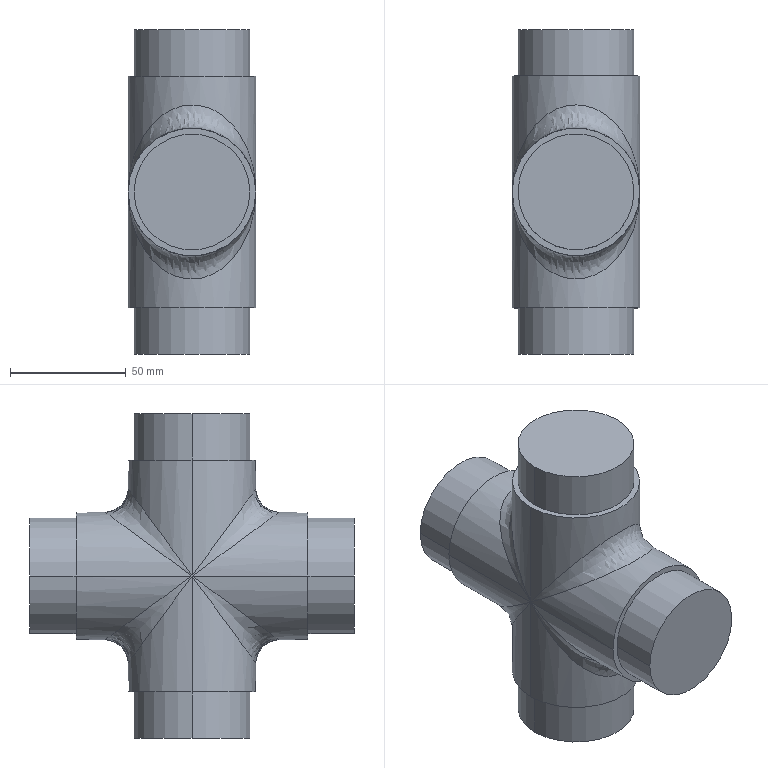Part | SolidWorks | 1 solid | 28 faces | box 55 x 140 x 140 mm | volume 524256 mm3 | cylinder 16 | plane 8 | spline 4 | commonest cylinder face diameters 50 x8 55 x8
STEP:
#1=CARTESIAN_POINT('',(-25.,-70.,0.));
#2=VERTEX_POINT('',#1);
#3=CARTESIAN_POINT('',(25.,-70.,0.));
#4=VERTEX_POINT('',#3);
#5=CARTESIAN_POINT('',(0.,-70.,0.));
#6=DIRECTION('',(0.,1.,0.));
#7=DIRECTION('',(-1.,0.,0.));
#8=AXIS2_PLACEMENT_3D('',#5,#6,#7);
#9=CIRCLE('',#8,25.);
#10=EDGE_CURVE('',#2,#4,#9,.T.);
#11=ORIENTED_EDGE('',*,*,#10,.T.);
#12=CARTESIAN_POINT('',(25.,-50.,0.));
#13=VERTEX_POINT('',#12);
#14=CARTESIAN_POINT('',(25.,70.,0.));
#15=DIRECTION('',(0.,1.,0.));
#16=VECTOR('',#15,1000.);
#17=LINE('',#14,#16);
#18=EDGE_CURVE('',#4,#13,#17,.T.);
#19=ORIENTED_EDGE('',*,*,#18,.T.);
#20=CARTESIAN_POINT('',(-25.,-50.,0.));
#21=VERTEX_POINT('',#20);
#22=CARTESIAN_POINT('',(0.,-50.,0.));
#23=DIRECTION('',(0.,1.,0.));
#24=DIRECTION('',(-1.,0.,0.));
#25=AXIS2_PLACEMENT_3D('',#22,#23,#24);
#26=CIRCLE('',#25,25.);
#27=EDGE_CURVE('',#21,#13,#26,.T.);
#28=ORIENTED_EDGE('',*,*,#27,.F.);
#29=CARTESIAN_POINT('',(-25.,70.,0.));
#30=DIRECTION('',(0.,1.,0.));
#31=VECTOR('',#30,1000.);
#32=LINE('',#29,#31);
#33=EDGE_CURVE('',#2,#21,#32,.T.);
#34=ORIENTED_EDGE('',*,*,#33,.F.);
#35=EDGE_LOOP('',(#11,#19,#28,#34));
#36=FACE_OUTER_BOUND('',#35,.T.);
#37=CARTESIAN_POINT('',(0.,70.,0.));
#38=DIRECTION('',(0.,1.,0.));
#39=DIRECTION('',(-1.,0.,0.));
#40=AXIS2_PLACEMENT_3D('',#37,#38,#39);
#41=CYLINDRICAL_SURFACE('',#40,25.);
#42=ADVANCED_FACE('',(#36),#41,.T.);
#43=CARTESIAN_POINT('',(-27.5,-50.,0.));
#44=VERTEX_POINT('',#43);
#45=CARTESIAN_POINT('',(27.5,-50.,0.));
#46=VERTEX_POINT('',#45);
#47=CARTESIAN_POINT('',(0.,-50.,0.));
#48=DIRECTION('',(0.,1.,0.));
#49=DIRECTION('',(-1.,0.,0.));
#50=AXIS2_PLACEMENT_3D('',#47,#48,#49);
#51=CIRCLE('',#50,27.5);
#52=EDGE_CURVE('',#44,#46,#51,.T.);
#53=ORIENTED_EDGE('',*,*,#52,.T.);
#54=CARTESIAN_POINT('',(27.5,0.,0.));
#55=VERTEX_POINT('',#54);
#56=CARTESIAN_POINT('',(27.5,70.,0.));
#57=DIRECTION('',(0.,1.,0.));
#58=VECTOR('',#57,1000.);
#59=LINE('',#56,#58);
#60=EDGE_CURVE('',#46,#55,#59,.T.);
#61=ORIENTED_EDGE('',*,*,#60,.T.);
#62=CARTESIAN_POINT('',(-27.5,0.,0.));
#63=VERTEX_POINT('',#62);
#64=CARTESIAN_POINT('',(27.5,0.,0.));
#65=CARTESIAN_POINT('',(27.5,-75.,55.));
#66=CARTESIAN_POINT('',(-27.5,-75.,55.));
#67=CARTESIAN_POINT('',(-27.5,0.,0.));
#68=(BOUNDED_CURVE()B_SPLINE_CURVE(3,(#64,#65,#66,#67),.UNSPECIFIED.,.F.,.F.)B_SPLINE_CURVE_WITH_KNOTS((4,4),(1.571,4.712),.UNSPECIFIED.)CURVE()GEOMETRIC_REPRESENTATION_ITEM()RATIONAL_B_SPLINE_CURVE((1.,0.3333,0.3333,1.))REPRESENTATION_ITEM(''));
#69=EDGE_CURVE('',#55,#63,#68,.T.);
#70=ORIENTED_EDGE('',*,*,#69,.T.);
#71=CARTESIAN_POINT('',(-27.5,70.,0.));
#72=DIRECTION('',(0.,1.,0.));
#73=VECTOR('',#72,1000.);
#74=LINE('',#71,#73);
#75=EDGE_CURVE('',#44,#63,#74,.T.);
#76=ORIENTED_EDGE('',*,*,#75,.F.);
#77=EDGE_LOOP('',(#53,#61,#70,#76));
#78=FACE_OUTER_BOUND('',#77,.T.);
#79=CARTESIAN_POINT('',(0.,70.,0.));
#80=DIRECTION('',(0.,1.,0.));
#81=DIRECTION('',(-1.,0.,0.));
#82=AXIS2_PLACEMENT_3D('',#79,#80,#81);
#83=CYLINDRICAL_SURFACE('',#82,27.5);
#84=ADVANCED_FACE('',(#78),#83,.T.);
#85=CARTESIAN_POINT('',(-27.5,0.,0.));
#86=CARTESIAN_POINT('',(-27.5,55.,-75.));
#87=CARTESIAN_POINT('',(27.5,55.,-75.));
#88=CARTESIAN_POINT('',(27.5,0.,0.));
#89=(BOUNDED_CURVE()B_SPLINE_CURVE(3,(#85,#86,#87,#88),.UNSPECIFIED.,.F.,.F.)B_SPLINE_CURVE_WITH_KNOTS((4,4),(4.712,7.854),.UNSPECIFIED.)CURVE()GEOMETRIC_REPRESENTATION_ITEM()RATIONAL_B_SPLINE_CURVE((1.,0.3333,0.3333,1.))REPRESENTATION_ITEM(''));
#90=EDGE_CURVE('',#63,#55,#89,.T.);
#91=ORIENTED_EDGE('',*,*,#90,.T.);
#92=CARTESIAN_POINT('',(27.5,0.,-50.));
#93=VERTEX_POINT('',#92);
#94=CARTESIAN_POINT('',(27.5,0.,50.));
#95=DIRECTION('',(0.,0.,-1.));
#96=VECTOR('',#95,1000.);
#97=LINE('',#94,#96);
#98=EDGE_CURVE('',#55,#93,#97,.T.);
#99=ORIENTED_EDGE('',*,*,#98,.T.);
#100=CARTESIAN_POINT('',(-27.5,0.,-50.));
#101=VERTEX_POINT('',#100);
#102=CARTESIAN_POINT('',(0.,0.,-50.));
#103=DIRECTION('',(0.,0.,1.));
#104=DIRECTION('',(1.,0.,0.));
#105=AXIS2_PLACEMENT_3D('',#102,#103,#104);
#106=CIRCLE('',#105,27.5);
#107=EDGE_CURVE('',#93,#101,#106,.T.);
#108=ORIENTED_EDGE('',*,*,#107,.T.);
#109=CARTESIAN_POINT('',(-27.5,0.,50.));
#110=DIRECTION('',(0.,0.,-1.));
#111=VECTOR('',#110,1000.);
#112=LINE('',#109,#111);
#113=EDGE_CURVE('',#63,#101,#112,.T.);
#114=ORIENTED_EDGE('',*,*,#113,.F.);
#115=EDGE_LOOP('',(#91,#99,#108,#114));
#116=FACE_OUTER_BOUND('',#115,.T.);
#117=CARTESIAN_POINT('',(0.,0.,50.));
#118=DIRECTION('',(0.,0.,-1.));
#119=DIRECTION('',(-1.,0.,0.));
#120=AXIS2_PLACEMENT_3D('',#117,#118,#119);
#121=CYLINDRICAL_SURFACE('',#120,27.5);
#122=ADVANCED_FACE('',(#116),#121,.T.);
#123=CARTESIAN_POINT('',(25.,0.,-50.));
#124=VERTEX_POINT('',#123);
#125=CARTESIAN_POINT('',(-25.,0.,-50.));
#126=VERTEX_POINT('',#125);
#127=CARTESIAN_POINT('',(0.,0.,-50.));
#128=DIRECTION('',(0.,0.,1.));
#129=DIRECTION('',(1.,0.,0.));
#130=AXIS2_PLACEMENT_3D('',#127,#128,#129);
#131=CIRCLE('',#130,25.);
#132=EDGE_CURVE('',#124,#126,#131,.T.);
#133=ORIENTED_EDGE('',*,*,#132,.F.);
#134=CARTESIAN_POINT('',(25.,0.,-70.));
#135=VERTEX_POINT('',#134);
#136=CARTESIAN_POINT('',(25.,0.,70.));
#137=DIRECTION('',(0.,0.,-1.));
#138=VECTOR('',#137,1000.);
#139=LINE('',#136,#138);
#140=EDGE_CURVE('',#124,#135,#139,.T.);
#141=ORIENTED_EDGE('',*,*,#140,.T.);
#142=CARTESIAN_POINT('',(-25.,0.,-70.));
#143=VERTEX_POINT('',#142);
#144=CARTESIAN_POINT('',(0.,0.,-70.));
#145=DIRECTION('',(0.,0.,1.));
#146=DIRECTION('',(1.,0.,0.));
#147=AXIS2_PLACEMENT_3D('',#144,#145,#146);
#148=CIRCLE('',#147,25.);
#149=EDGE_CURVE('',#135,#143,#148,.T.);
#150=ORIENTED_EDGE('',*,*,#149,.T.);
#151=CARTESIAN_POINT('',(-25.,0.,70.));
#152=DIRECTION('',(0.,0.,-1.));
#153=VECTOR('',#152,1000.);
#154=LINE('',#151,#153);
#155=EDGE_CURVE('',#126,#143,#154,.T.);
#156=ORIENTED_EDGE('',*,*,#155,.F.);
#157=EDGE_LOOP('',(#133,#141,#150,#156));
#158=FACE_OUTER_BOUND('',#157,.T.);
#159=CARTESIAN_POINT('',(0.,0.,70.));
#160=DIRECTION('',(0.,0.,-1.));
#161=DIRECTION('',(-1.,0.,0.));
#162=AXIS2_PLACEMENT_3D('',#159,#160,#161);
#163=CYLINDRICAL_SURFACE('',#162,25.);
#164=ADVANCED_FACE('',(#158),#163,.T.);
#165=CARTESIAN_POINT('',(-27.5,0.,0.));
#166=CARTESIAN_POINT('',(-27.5,75.,55.));
#167=CARTESIAN_POINT('',(27.5,75.,55.));
#168=CARTESIAN_POINT('',(27.5,0.,0.));
#169=(BOUNDED_CURVE()B_SPLINE_CURVE(3,(#165,#166,#167,#168),.UNSPECIFIED.,.F.,.T.)B_SPLINE_CURVE_WITH_KNOTS((4,4),(4.712,7.854),.UNSPECIFIED.)CURVE()GEOMETRIC_REPRESENTATION_ITEM()RATIONAL_B_SPLINE_CURVE((1.,0.3333,0.3333,1.))REPRESENTATION_ITEM(''));
#170=EDGE_CURVE('',#63,#55,#169,.T.);
#171=ORIENTED_EDGE('',*,*,#170,.T.);
#172=CARTESIAN_POINT('',(27.5,50.,0.));
#173=VERTEX_POINT('',#172);
#174=CARTESIAN_POINT('',(27.5,70.,0.));
#175=DIRECTION('',(0.,1.,0.));
#176=VECTOR('',#175,1000.);
#177=LINE('',#174,#176);
#178=EDGE_CURVE('',#55,#173,#177,.T.);
#179=ORIENTED_EDGE('',*,*,#178,.T.);
#180=CARTESIAN_POINT('',(-27.5,50.,0.));
#181=VERTEX_POINT('',#180);
#182=CARTESIAN_POINT('',(0.,50.,0.));
#183=DIRECTION('',(0.,1.,0.));
#184=DIRECTION('',(-1.,0.,0.));
#185=AXIS2_PLACEMENT_3D('',#182,#183,#184);
#186=CIRCLE('',#185,27.5);
#187=EDGE_CURVE('',#181,#173,#186,.T.);
#188=ORIENTED_EDGE('',*,*,#187,.F.);
#189=CARTESIAN_POINT('',(-27.5,70.,0.));
#190=DIRECTION('',(0.,1.,0.));
#191=VECTOR('',#190,1000.);
#192=LINE('',#189,#191);
#193=EDGE_CURVE('',#63,#181,#192,.T.);
#194=ORIENTED_EDGE('',*,*,#193,.F.);
#195=EDGE_LOOP('',(#171,#179,#188,#194));
#196=FACE_OUTER_BOUND('',#195,.T.);
#197=CARTESIAN_POINT('',(0.,70.,0.));
#198=DIRECTION('',(0.,1.,0.));
#199=DIRECTION('',(-1.,0.,0.));
#200=AXIS2_PLACEMENT_3D('',#197,#198,#199);
#201=CYLINDRICAL_SURFACE('',#200,27.5);
#202=ADVANCED_FACE('',(#196),#201,.T.);
#203=CARTESIAN_POINT('',(-25.,50.,0.));
#204=VERTEX_POINT('',#203);
#205=CARTESIAN_POINT('',(25.,50.,0.));
#206=VERTEX_POINT('',#205);
#207=CARTESIAN_POINT('',(0.,50.,0.));
#208=DIRECTION('',(0.,1.,0.));
#209=DIRECTION('',(-1.,0.,0.));
#210=AXIS2_PLACEMENT_3D('',#207,#208,#209);
#211=CIRCLE('',#210,25.);
#212=EDGE_CURVE('',#204,#206,#211,.T.);
#213=ORIENTED_EDGE('',*,*,#212,.T.);
#214=CARTESIAN_POINT('',(25.,70.,0.));
#215=VERTEX_POINT('',#214);
#216=CARTESIAN_POINT('',(25.,70.,0.));
#217=DIRECTION('',(0.,1.,0.));
#218=VECTOR('',#217,1000.);
#219=LINE('',#216,#218);
#220=EDGE_CURVE('',#206,#215,#219,.T.);
#221=ORIENTED_EDGE('',*,*,#220,.T.);
#222=CARTESIAN_POINT('',(-25.,70.,0.));
#223=VERTEX_POINT('',#222);
#224=CARTESIAN_POINT('',(0.,70.,0.));
#225=DIRECTION('',(0.,1.,0.));
#226=DIRECTION('',(-1.,0.,0.));
#227=AXIS2_PLACEMENT_3D('',#224,#225,#226);
#228=CIRCLE('',#227,25.);
#229=EDGE_CURVE('',#223,#215,#228,.T.);
#230=ORIENTED_EDGE('',*,*,#229,.F.);
#231=CARTESIAN_POINT('',(-25.,70.,0.));
#232=DIRECTION('',(0.,1.,0.));
#233=VECTOR('',#232,1000.);
#234=LINE('',#231,#233);
#235=EDGE_CURVE('',#204,#223,#234,.T.);
#236=ORIENTED_EDGE('',*,*,#235,.F.);
#237=EDGE_LOOP('',(#213,#221,#230,#236));
#238=FACE_OUTER_BOUND('',#237,.T.);
#239=CARTESIAN_POINT('',(0.,70.,0.));
#240=DIRECTION('',(0.,1.,0.));
#241=DIRECTION('',(-1.,0.,0.));
#242=AXIS2_PLACEMENT_3D('',#239,#240,#241);
#243=CYLINDRICAL_SURFACE('',#242,25.);
#244=ADVANCED_FACE('',(#238),#243,.T.);
#245=CARTESIAN_POINT('',(25.,0.,70.));
#246=VERTEX_POINT('',#245);
#247=CARTESIAN_POINT('',(-25.,0.,70.));
#248=VERTEX_POINT('',#247);
#249=CARTESIAN_POINT('',(0.,0.,70.));
#250=DIRECTION('',(0.,0.,1.));
#251=DIRECTION('',(1.,0.,0.));
#252=AXIS2_PLACEMENT_3D('',#249,#250,#251);
#253=CIRCLE('',#252,25.);
#254=EDGE_CURVE('',#246,#248,#253,.T.);
#255=ORIENTED_EDGE('',*,*,#254,.F.);
#256=CARTESIAN_POINT('',(25.,0.,50.));
#257=VERTEX_POINT('',#256);
#258=CARTESIAN_POINT('',(25.,0.,70.));
#259=DIRECTION('',(0.,0.,-1.));
#260=VECTOR('',#259,1000.);
#261=LINE('',#258,#260);
#262=EDGE_CURVE('',#246,#257,#261,.T.);
#263=ORIENTED_EDGE('',*,*,#262,.T.);
#264=CARTESIAN_POINT('',(-25.,0.,50.));
#265=VERTEX_POINT('',#264);
#266=CARTESIAN_POINT('',(0.,0.,50.));
#267=DIRECTION('',(0.,0.,1.));
#268=DIRECTION('',(1.,0.,0.));
#269=AXIS2_PLACEMENT_3D('',#266,#267,#268);
#270=CIRCLE('',#269,25.);
#271=EDGE_CURVE('',#257,#265,#270,.T.);
#272=ORIENTED_EDGE('',*,*,#271,.T.);
#273=CARTESIAN_POINT('',(-25.,0.,70.));
#274=DIRECTION('',(0.,0.,-1.));
#275=VECTOR('',#274,1000.);
#276=LINE('',#273,#275);
#277=EDGE_CURVE('',#248,#265,#276,.T.);
#278=ORIENTED_EDGE('',*,*,#277,.F.);
#279=EDGE_LOOP('',(#255,#263,#272,#278));
#280=FACE_OUTER_BOUND('',#279,.T.);
#281=CARTESIAN_POINT('',(0.,0.,70.));
#282=DIRECTION('',(0.,0.,-1.));
#283=DIRECTION('',(-1.,0.,0.));
#284=AXIS2_PLACEMENT_3D('',#281,#282,#283);
#285=CYLINDRICAL_SURFACE('',#284,25.);
#286=ADVANCED_FACE('',(#280),#285,.T.);
#287=CARTESIAN_POINT('',(27.5,0.,50.));
#288=VERTEX_POINT('',#287);
#289=CARTESIAN_POINT('',(-27.5,0.,50.));
#290=VERTEX_POINT('',#289);
#291=CARTESIAN_POINT('',(0.,0.,50.));
#292=DIRECTION('',(0.,0.,1.));
#293=DIRECTION('',(1.,0.,0.));
#294=AXIS2_PLACEMENT_3D('',#291,#292,#293);
#295=CIRCLE('',#294,27.5);
#296=EDGE_CURVE('',#288,#290,#295,.T.);
#297=ORIENTED_EDGE('',*,*,#296,.F.);
#298=CARTESIAN_POINT('',(27.5,0.,50.));
#299=DIRECTION('',(0.,0.,-1.));
#300=VECTOR('',#299,1000.);
#301=LINE('',#298,#300);
#302=EDGE_CURVE('',#288,#55,#301,.T.);
#303=ORIENTED_EDGE('',*,*,#302,.T.);
#304=CARTESIAN_POINT('',(27.5,0.,0.));
#305=CARTESIAN_POINT('',(27.5,55.,75.));
#306=CARTESIAN_POINT('',(-27.5,55.,75.));
#307=CARTESIAN_POINT('',(-27.5,0.,0.));
#308=(BOUNDED_CURVE()B_SPLINE_CURVE(3,(#304,#305,#306,#307),.UNSPECIFIED.,.F.,.F.)B_SPLINE_CURVE_WITH_KNOTS((4,4),(4.712,7.854),.UNSPECIFIED.)CURVE()GEOMETRIC_REPRESENTATION_ITEM()RATIONAL_B_SPLINE_CURVE((1.,0.3333,0.3333,1.))REPRESENTATION_ITEM(''));
#309=EDGE_CURVE('',#55,#63,#308,.T.);
#310=ORIENTED_EDGE('',*,*,#309,.T.);
#311=CARTESIAN_POINT('',(-27.5,0.,50.));
#312=DIRECTION('',(0.,0.,-1.));
#313=VECTOR('',#312,1000.);
#314=LINE('',#311,#313);
#315=EDGE_CURVE('',#290,#63,#314,.T.);
#316=ORIENTED_EDGE('',*,*,#315,.F.);
#317=EDGE_LOOP('',(#297,#303,#310,#316));
#318=FACE_OUTER_BOUND('',#317,.T.);
#319=CARTESIAN_POINT('',(0.,0.,50.));
#320=DIRECTION('',(0.,0.,-1.));
#321=DIRECTION('',(-1.,0.,0.));
#322=AXIS2_PLACEMENT_3D('',#319,#320,#321);
#323=CYLINDRICAL_SURFACE('',#322,27.5);
#324=ADVANCED_FACE('',(#318),#323,.T.);
#325=ORIENTED_EDGE('',*,*,#302,.F.);
#326=CARTESIAN_POINT('',(0.,0.,50.));
#327=DIRECTION('',(0.,0.,1.));
#328=DIRECTION('',(1.,0.,0.));
#329=AXIS2_PLACEMENT_3D('',#326,#327,#328);
#330=CIRCLE('',#329,27.5);
#331=EDGE_CURVE('',#290,#288,#330,.T.);
#332=ORIENTED_EDGE('',*,*,#331,.F.);
#333=ORIENTED_EDGE('',*,*,#315,.T.);
#334=CARTESIAN_POINT('',(-27.5,0.,0.));
#335=CARTESIAN_POINT('',(-27.5,-55.,75.));
#336=CARTESIAN_POINT('',(27.5,-55.,75.));
#337=CARTESIAN_POINT('',(27.5,0.,0.));
#338=(BOUNDED_CURVE()B_SPLINE_CURVE(3,(#334,#335,#336,#337),.UNSPECIFIED.,.F.,.F.)B_SPLINE_CURVE_WITH_KNOTS((4,4),(1.571,4.712),.UNSPECIFIED.)CURVE()GEOMETRIC_REPRESENTATION_ITEM()RATIONAL_B_SPLINE_CURVE((1.,0.3333,0.3333,1.))REPRESENTATION_ITEM(''));
#339=EDGE_CURVE('',#63,#55,#338,.T.);
#340=ORIENTED_EDGE('',*,*,#339,.T.);
#341=EDGE_LOOP('',(#325,#332,#333,#340));
#342=FACE_OUTER_BOUND('',#341,.T.);
#343=CARTESIAN_POINT('',(0.,0.,50.));
#344=DIRECTION('',(0.,0.,-1.));
#345=DIRECTION('',(-1.,0.,0.));
#346=AXIS2_PLACEMENT_3D('',#343,#344,#345);
#347=CYLINDRICAL_SURFACE('',#346,27.5);
#348=ADVANCED_FACE('',(#342),#347,.T.);
#349=ORIENTED_EDGE('',*,*,#262,.F.);
#350=CARTESIAN_POINT('',(0.,0.,70.));
#351=DIRECTION('',(0.,0.,1.));
#352=DIRECTION('',(1.,0.,0.));
#353=AXIS2_PLACEMENT_3D('',#350,#351,#352);
#354=CIRCLE('',#353,25.);
#355=EDGE_CURVE('',#248,#246,#354,.T.);
#356=ORIENTED_EDGE('',*,*,#355,.F.);
#357=ORIENTED_EDGE('',*,*,#277,.T.);
#358=CARTESIAN_POINT('',(0.,0.,50.));
#359=DIRECTION('',(0.,0.,1.));
#360=DIRECTION('',(1.,0.,0.));
#361=AXIS2_PLACEMENT_3D('',#358,#359,#360);
#362=CIRCLE('',#361,25.);
#363=EDGE_CURVE('',#265,#257,#362,.T.);
#364=ORIENTED_EDGE('',*,*,#363,.T.);
#365=EDGE_LOOP('',(#349,#356,#357,#364));
#366=FACE_OUTER_BOUND('',#365,.T.);
#367=CARTESIAN_POINT('',(0.,0.,70.));
#368=DIRECTION('',(0.,0.,-1.));
#369=DIRECTION('',(-1.,0.,0.));
#370=AXIS2_PLACEMENT_3D('',#367,#368,#369);
#371=CYLINDRICAL_SURFACE('',#370,25.);
#372=ADVANCED_FACE('',(#366),#371,.T.);
#373=ORIENTED_EDGE('',*,*,#355,.T.);
#374=ORIENTED_EDGE('',*,*,#254,.T.);
#375=EDGE_LOOP('',(#373,#374));
#376=FACE_OUTER_BOUND('',#375,.T.);
#377=CARTESIAN_POINT('',(0.,0.,70.));
#378=DIRECTION('',(0.,0.,1.));
#379=DIRECTION('',(1.,0.,0.));
#380=AXIS2_PLACEMENT_3D('',#377,#378,#379);
#381=PLANE('',#380);
#382=ADVANCED_FACE('',(#376),#381,.T.);
#383=ORIENTED_EDGE('',*,*,#363,.F.);
#384=ORIENTED_EDGE('',*,*,#271,.F.);
#385=EDGE_LOOP('',(#383,#384));
#386=FACE_BOUND('',#385,.T.);
#387=ORIENTED_EDGE('',*,*,#331,.T.);
#388=ORIENTED_EDGE('',*,*,#296,.T.);
#389=EDGE_LOOP('',(#387,#388));
#390=FACE_OUTER_BOUND('',#389,.T.);
#391=CARTESIAN_POINT('',(0.,0.,50.));
#392=DIRECTION('',(0.,0.,1.));
#393=DIRECTION('',(1.,0.,0.));
#394=AXIS2_PLACEMENT_3D('',#391,#392,#393);
#395=PLANE('',#394);
#396=ADVANCED_FACE('',(#386,#390),#395,.T.);
#397=ORIENTED_EDGE('',*,*,#229,.T.);
#398=CARTESIAN_POINT('',(0.,70.,0.));
#399=DIRECTION('',(0.,1.,0.));
#400=DIRECTION('',(-1.,0.,0.));
#401=AXIS2_PLACEMENT_3D('',#398,#399,#400);
#402=CIRCLE('',#401,25.);
#403=EDGE_CURVE('',#215,#223,#402,.T.);
#404=ORIENTED_EDGE('',*,*,#403,.T.);
#405=EDGE_LOOP('',(#397,#404));
#406=FACE_OUTER_BOUND('',#405,.T.);
#407=CARTESIAN_POINT('',(0.,70.,0.));
#408=DIRECTION('',(0.,-1.,0.));
#409=DIRECTION('',(1.,0.,0.));
#410=AXIS2_PLACEMENT_3D('',#407,#408,#409);
#411=PLANE('',#410);
#412=ADVANCED_FACE('',(#406),#411,.F.);
#413=ORIENTED_EDGE('',*,*,#220,.F.);
#414=CARTESIAN_POINT('',(0.,50.,0.));
#415=DIRECTION('',(0.,1.,0.));
#416=DIRECTION('',(-1.,0.,0.));
#417=AXIS2_PLACEMENT_3D('',#414,#415,#416);
#418=CIRCLE('',#417,25.);
#419=EDGE_CURVE('',#206,#204,#418,.T.);
#420=ORIENTED_EDGE('',*,*,#419,.T.);
#421=ORIENTED_EDGE('',*,*,#235,.T.);
#422=ORIENTED_EDGE('',*,*,#403,.F.);
#423=EDGE_LOOP('',(#413,#420,#421,#422));
#424=FACE_OUTER_BOUND('',#423,.T.);
#425=CARTESIAN_POINT('',(0.,70.,0.));
#426=DIRECTION('',(0.,1.,0.));
#427=DIRECTION('',(-1.,0.,0.));
#428=AXIS2_PLACEMENT_3D('',#425,#426,#427);
#429=CYLINDRICAL_SURFACE('',#428,25.);
#430=ADVANCED_FACE('',(#424),#429,.T.);
#431=ORIENTED_EDGE('',*,*,#212,.F.);
#432=ORIENTED_EDGE('',*,*,#419,.F.);
#433=EDGE_LOOP('',(#431,#432));
#434=FACE_BOUND('',#433,.T.);
#435=ORIENTED_EDGE('',*,*,#187,.T.);
#436=CARTESIAN_POINT('',(0.,50.,0.));
#437=DIRECTION('',(0.,1.,0.));
#438=DIRECTION('',(-1.,0.,0.));
#439=AXIS2_PLACEMENT_3D('',#436,#437,#438);
#440=CIRCLE('',#439,27.5);
#441=EDGE_CURVE('',#173,#181,#440,.T.);
#442=ORIENTED_EDGE('',*,*,#441,.T.);
#443=EDGE_LOOP('',(#435,#442));
#444=FACE_OUTER_BOUND('',#443,.T.);
#445=CARTESIAN_POINT('',(25.,50.,0.));
#446=DIRECTION('',(0.,-1.,0.));
#447=DIRECTION('',(1.,0.,0.));
#448=AXIS2_PLACEMENT_3D('',#445,#446,#447);
#449=PLANE('',#448);
#450=ADVANCED_FACE('',(#434,#444),#449,.F.);
#451=ORIENTED_EDGE('',*,*,#178,.F.);
#452=CARTESIAN_POINT('',(27.5,0.,0.));
#453=CARTESIAN_POINT('',(27.5,75.,-55.));
#454=CARTESIAN_POINT('',(-27.5,75.,-55.));
#455=CARTESIAN_POINT('',(-27.5,0.,0.));
#456=(BOUNDED_CURVE()B_SPLINE_CURVE(3,(#452,#453,#454,#455),.UNSPECIFIED.,.F.,.T.)B_SPLINE_CURVE_WITH_KNOTS((4,4),(4.712,7.854),.UNSPECIFIED.)CURVE()GEOMETRIC_REPRESENTATION_ITEM()RATIONAL_B_SPLINE_CURVE((1.,0.3333,0.3333,1.))REPRESENTATION_ITEM(''));
#457=EDGE_CURVE('',#55,#63,#456,.T.);
#458=ORIENTED_EDGE('',*,*,#457,.T.);
#459=ORIENTED_EDGE('',*,*,#193,.T.);
#460=ORIENTED_EDGE('',*,*,#441,.F.);
#461=EDGE_LOOP('',(#451,#458,#459,#460));
#462=FACE_OUTER_BOUND('',#461,.T.);
#463=CARTESIAN_POINT('',(0.,70.,0.));
#464=DIRECTION('',(0.,1.,0.));
#465=DIRECTION('',(-1.,0.,0.));
#466=AXIS2_PLACEMENT_3D('',#463,#464,#465);
#467=CYLINDRICAL_SURFACE('',#466,27.5);
#468=ADVANCED_FACE('',(#462),#467,.T.);
#469=CARTESIAN_POINT('',(0.,0.,-70.));
#470=DIRECTION('',(0.,0.,1.));
#471=DIRECTION('',(1.,0.,0.));
#472=AXIS2_PLACEMENT_3D('',#469,#470,#471);
#473=CIRCLE('',#472,25.);
#474=EDGE_CURVE('',#143,#135,#473,.T.);
#475=ORIENTED_EDGE('',*,*,#474,.F.);
#476=ORIENTED_EDGE('',*,*,#149,.F.);
#477=EDGE_LOOP('',(#475,#476));
#478=FACE_OUTER_BOUND('',#477,.T.);
#479=CARTESIAN_POINT('',(0.,0.,-70.));
#480=DIRECTION('',(0.,0.,1.));
#481=DIRECTION('',(1.,0.,0.));
#482=AXIS2_PLACEMENT_3D('',#479,#480,#481);
#483=PLANE('',#482);
#484=ADVANCED_FACE('',(#478),#483,.F.);
#485=ORIENTED_EDGE('',*,*,#140,.F.);
#486=CARTESIAN_POINT('',(0.,0.,-50.));
#487=DIRECTION('',(0.,0.,1.));
#488=DIRECTION('',(1.,0.,0.));
#489=AXIS2_PLACEMENT_3D('',#486,#487,#488);
#490=CIRCLE('',#489,25.);
#491=EDGE_CURVE('',#126,#124,#490,.T.);
#492=ORIENTED_EDGE('',*,*,#491,.F.);
#493=ORIENTED_EDGE('',*,*,#155,.T.);
#494=ORIENTED_EDGE('',*,*,#474,.T.);
#495=EDGE_LOOP('',(#485,#492,#493,#494));
#496=FACE_OUTER_BOUND('',#495,.T.);
#497=CARTESIAN_POINT('',(0.,0.,70.));
#498=DIRECTION('',(0.,0.,-1.));
#499=DIRECTION('',(-1.,0.,0.));
#500=AXIS2_PLACEMENT_3D('',#497,#498,#499);
#501=CYLINDRICAL_SURFACE('',#500,25.);
#502=ADVANCED_FACE('',(#496),#501,.T.);
#503=ORIENTED_EDGE('',*,*,#491,.T.);
#504=ORIENTED_EDGE('',*,*,#132,.T.);
#505=EDGE_LOOP('',(#503,#504));
#506=FACE_BOUND('',#505,.T.);
#507=CARTESIAN_POINT('',(0.,0.,-50.));
#508=DIRECTION('',(0.,0.,1.));
#509=DIRECTION('',(1.,0.,0.));
#510=AXIS2_PLACEMENT_3D('',#507,#508,#509);
#511=CIRCLE('',#510,27.5);
#512=EDGE_CURVE('',#101,#93,#511,.T.);
#513=ORIENTED_EDGE('',*,*,#512,.F.);
#514=ORIENTED_EDGE('',*,*,#107,.F.);
#515=EDGE_LOOP('',(#513,#514));
#516=FACE_OUTER_BOUND('',#515,.T.);
#517=CARTESIAN_POINT('',(0.,0.,-50.));
#518=DIRECTION('',(0.,0.,1.));
#519=DIRECTION('',(1.,0.,0.));
#520=AXIS2_PLACEMENT_3D('',#517,#518,#519);
#521=PLANE('',#520);
#522=ADVANCED_FACE('',(#506,#516),#521,.F.);
#523=ORIENTED_EDGE('',*,*,#98,.F.);
#524=CARTESIAN_POINT('',(27.5,0.,0.));
#525=CARTESIAN_POINT('',(27.5,-55.,-75.));
#526=CARTESIAN_POINT('',(-27.5,-55.,-75.));
#527=CARTESIAN_POINT('',(-27.5,0.,0.));
#528=(BOUNDED_CURVE()B_SPLINE_CURVE(3,(#524,#525,#526,#527),.UNSPECIFIED.,.F.,.T.)B_SPLINE_CURVE_WITH_KNOTS((4,4),(1.571,4.712),.UNSPECIFIED.)CURVE()GEOMETRIC_REPRESENTATION_ITEM()RATIONAL_B_SPLINE_CURVE((1.,0.3333,0.3333,1.))REPRESENTATION_ITEM(''));
#529=EDGE_CURVE('',#55,#63,#528,.T.);
#530=ORIENTED_EDGE('',*,*,#529,.T.);
#531=ORIENTED_EDGE('',*,*,#113,.T.);
#532=ORIENTED_EDGE('',*,*,#512,.T.);
#533=EDGE_LOOP('',(#523,#530,#531,#532));
#534=FACE_OUTER_BOUND('',#533,.T.);
#535=CARTESIAN_POINT('',(0.,0.,50.));
#536=DIRECTION('',(0.,0.,-1.));
#537=DIRECTION('',(-1.,0.,0.));
#538=AXIS2_PLACEMENT_3D('',#535,#536,#537);
#539=CYLINDRICAL_SURFACE('',#538,27.5);
#540=ADVANCED_FACE('',(#534),#539,.T.);
#541=ORIENTED_EDGE('',*,*,#60,.F.);
#542=CARTESIAN_POINT('',(0.,-50.,0.));
#543=DIRECTION('',(0.,1.,0.));
#544=DIRECTION('',(-1.,0.,0.));
#545=AXIS2_PLACEMENT_3D('',#542,#543,#544);
#546=CIRCLE('',#545,27.5);
#547=EDGE_CURVE('',#46,#44,#546,.T.);
#548=ORIENTED_EDGE('',*,*,#547,.T.);
#549=ORIENTED_EDGE('',*,*,#75,.T.);
#550=CARTESIAN_POINT('',(-27.5,0.,0.));
#551=CARTESIAN_POINT('',(-27.5,-75.,-55.));
#552=CARTESIAN_POINT('',(27.5,-75.,-55.));
#553=CARTESIAN_POINT('',(27.5,0.,0.));
#554=(BOUNDED_CURVE()B_SPLINE_CURVE(3,(#550,#551,#552,#553),.UNSPECIFIED.,.F.,.F.)B_SPLINE_CURVE_WITH_KNOTS((4,4),(1.571,4.712),.UNSPECIFIED.)CURVE()GEOMETRIC_REPRESENTATION_ITEM()RATIONAL_B_SPLINE_CURVE((1.,0.3333,0.3333,1.))REPRESENTATION_ITEM(''));
#555=EDGE_CURVE('',#63,#55,#554,.T.);
#556=ORIENTED_EDGE('',*,*,#555,.T.);
#557=EDGE_LOOP('',(#541,#548,#549,#556));
#558=FACE_OUTER_BOUND('',#557,.T.);
#559=CARTESIAN_POINT('',(0.,70.,0.));
#560=DIRECTION('',(0.,1.,0.));
#561=DIRECTION('',(-1.,0.,0.));
#562=AXIS2_PLACEMENT_3D('',#559,#560,#561);
#563=CYLINDRICAL_SURFACE('',#562,27.5);
#564=ADVANCED_FACE('',(#558),#563,.T.);
#565=ORIENTED_EDGE('',*,*,#10,.F.);
#566=CARTESIAN_POINT('',(0.,-70.,0.));
#567=DIRECTION('',(0.,1.,0.));
#568=DIRECTION('',(-1.,0.,0.));
#569=AXIS2_PLACEMENT_3D('',#566,#567,#568);
#570=CIRCLE('',#569,25.);
#571=EDGE_CURVE('',#4,#2,#570,.T.);
#572=ORIENTED_EDGE('',*,*,#571,.F.);
#573=EDGE_LOOP('',(#565,#572));
#574=FACE_OUTER_BOUND('',#573,.T.);
#575=CARTESIAN_POINT('',(0.,-70.,0.));
#576=DIRECTION('',(0.,1.,0.));
#577=DIRECTION('',(-1.,0.,0.));
#578=AXIS2_PLACEMENT_3D('',#575,#576,#577);
#579=PLANE('',#578);
#580=ADVANCED_FACE('',(#574),#579,.F.);
#581=ORIENTED_EDGE('',*,*,#18,.F.);
#582=ORIENTED_EDGE('',*,*,#571,.T.);
#583=ORIENTED_EDGE('',*,*,#33,.T.);
#584=CARTESIAN_POINT('',(0.,-50.,0.));
#585=DIRECTION('',(0.,1.,0.));
#586=DIRECTION('',(-1.,0.,0.));
#587=AXIS2_PLACEMENT_3D('',#584,#585,#586);
#588=CIRCLE('',#587,25.);
#589=EDGE_CURVE('',#13,#21,#588,.T.);
#590=ORIENTED_EDGE('',*,*,#589,.F.);
#591=EDGE_LOOP('',(#581,#582,#583,#590));
#592=FACE_OUTER_BOUND('',#591,.T.);
#593=CARTESIAN_POINT('',(0.,70.,0.));
#594=DIRECTION('',(0.,1.,0.));
#595=DIRECTION('',(-1.,0.,0.));
#596=AXIS2_PLACEMENT_3D('',#593,#594,#595);
#597=CYLINDRICAL_SURFACE('',#596,25.);
#598=ADVANCED_FACE('',(#592),#597,.T.);
#599=ORIENTED_EDGE('',*,*,#52,.F.);
#600=ORIENTED_EDGE('',*,*,#547,.F.);
#601=EDGE_LOOP('',(#599,#600));
#602=FACE_OUTER_BOUND('',#601,.T.);
#603=ORIENTED_EDGE('',*,*,#27,.T.);
#604=ORIENTED_EDGE('',*,*,#589,.T.);
#605=EDGE_LOOP('',(#603,#604));
#606=FACE_BOUND('',#605,.T.);
#607=CARTESIAN_POINT('',(25.,-50.,0.));
#608=DIRECTION('',(0.,1.,0.));
#609=DIRECTION('',(-1.,0.,0.));
#610=AXIS2_PLACEMENT_3D('',#607,#608,#609);
#611=PLANE('',#610);
#612=ADVANCED_FACE('',(#602,#606),#611,.F.);
#613=ORIENTED_EDGE('',*,*,#170,.F.);
#614=ORIENTED_EDGE('',*,*,#309,.F.);
#615=EDGE_LOOP('',(#613,#614));
#616=FACE_OUTER_BOUND('',#615,.T.);
#617=CARTESIAN_POINT('',(-27.5,0.,0.));
#618=CARTESIAN_POINT('',(-27.5,0.,0.));
#619=CARTESIAN_POINT('',(-27.5,0.,0.));
#620=CARTESIAN_POINT('',(-27.5,2.454,1.8));
#621=CARTESIAN_POINT('',(-27.5,2.127,2.127));
#622=CARTESIAN_POINT('',(-27.5,1.8,2.454));
#623=CARTESIAN_POINT('',(-27.323,4.909,3.6));
#624=CARTESIAN_POINT('',(-27.255,4.267,4.267));
#625=CARTESIAN_POINT('',(-27.323,3.6,4.909));
#626=CARTESIAN_POINT('',(-26.62,9.723,7.13));
#627=CARTESIAN_POINT('',(-26.302,8.402,8.402));
#628=CARTESIAN_POINT('',(-26.62,7.13,9.723));
#629=CARTESIAN_POINT('',(-26.095,12.083,8.861));
#630=CARTESIAN_POINT('',(-25.583,10.42,10.42));
#631=CARTESIAN_POINT('',(-26.095,8.861,12.083));
#632=CARTESIAN_POINT('',(-24.718,16.618,12.187));
#633=CARTESIAN_POINT('',(-23.747,14.2,14.2));
#634=CARTESIAN_POINT('',(-24.718,12.187,16.618));
#635=CARTESIAN_POINT('',(-23.865,18.793,13.782));
#636=CARTESIAN_POINT('',(-22.611,15.976,15.976));
#637=CARTESIAN_POINT('',(-23.865,13.782,18.793));
#638=CARTESIAN_POINT('',(-21.865,22.875,16.775));
#639=CARTESIAN_POINT('',(-20.04,19.18,19.18));
#640=CARTESIAN_POINT('',(-21.865,16.775,22.875));
#641=CARTESIAN_POINT('',(-20.718,24.781,18.173));
#642=CARTESIAN_POINT('',(-18.586,20.607,20.607));
#643=CARTESIAN_POINT('',(-20.718,18.173,24.781));
#644=CARTESIAN_POINT('',(-18.173,28.252,20.718));
#645=CARTESIAN_POINT('',(-15.524,23.051,23.051));
#646=CARTESIAN_POINT('',(-18.173,20.718,28.252));
#647=CARTESIAN_POINT('',(-16.775,29.817,21.865));
#648=CARTESIAN_POINT('',(-13.908,24.052,24.052));
#649=CARTESIAN_POINT('',(-16.775,21.865,29.817));
#650=CARTESIAN_POINT('',(-14.53,31.862,23.365));
#651=CARTESIAN_POINT('',(-11.533,25.227,25.227));
#652=CARTESIAN_POINT('',(-14.53,23.365,31.862));
#653=CARTESIAN_POINT('',(-13.757,32.494,23.829));
#654=CARTESIAN_POINT('',(-10.737,25.568,25.568));
#655=CARTESIAN_POINT('',(-13.757,23.829,32.494));
#656=CARTESIAN_POINT('',(-12.17,33.651,24.677));
#657=CARTESIAN_POINT('',(-9.173,26.151,26.151));
#658=CARTESIAN_POINT('',(-12.17,24.677,33.651));
#659=CARTESIAN_POINT('',(-11.355,34.176,25.062));
#660=CARTESIAN_POINT('',(-8.408,26.391,26.391));
#661=CARTESIAN_POINT('',(-11.355,25.062,34.176));
#662=CARTESIAN_POINT('',(-9.692,35.115,25.751));
#663=CARTESIAN_POINT('',(-6.926,26.787,26.787));
#664=CARTESIAN_POINT('',(-9.692,25.751,35.115));
#665=CARTESIAN_POINT('',(-8.844,35.529,26.055));
#666=CARTESIAN_POINT('',(-6.212,26.94,26.94));
#667=CARTESIAN_POINT('',(-8.844,26.055,35.529));
#668=CARTESIAN_POINT('',(-7.122,36.241,26.577));
#669=CARTESIAN_POINT('',(-4.839,27.181,27.181));
#670=CARTESIAN_POINT('',(-7.122,26.577,36.241));
#671=CARTESIAN_POINT('',(-6.248,36.54,26.796));
#672=CARTESIAN_POINT('',(-4.184,27.268,27.268));
#673=CARTESIAN_POINT('',(-6.248,26.796,36.54));
#674=CARTESIAN_POINT('',(-4.482,37.019,27.147));
#675=CARTESIAN_POINT('',(-2.923,27.396,27.396));
#676=CARTESIAN_POINT('',(-4.482,27.147,37.019));
#677=CARTESIAN_POINT('',(-3.591,37.199,27.279));
#678=CARTESIAN_POINT('',(-2.321,27.436,27.436));
#679=CARTESIAN_POINT('',(-3.591,27.279,37.199));
#680=CARTESIAN_POINT('',(-1.8,37.44,27.456));
#681=CARTESIAN_POINT('',(-1.144,27.489,27.489));
#682=CARTESIAN_POINT('',(-1.8,27.456,37.44));
#683=CARTESIAN_POINT('',(-0.8999,37.5,27.5));
#684=CARTESIAN_POINT('',(-0.5727,27.5,27.5));
#685=CARTESIAN_POINT('',(-0.8999,27.5,37.5));
#686=CARTESIAN_POINT('',(0.8999,37.5,27.5));
#687=CARTESIAN_POINT('',(0.5727,27.5,27.5));
#688=CARTESIAN_POINT('',(0.8999,27.5,37.5));
#689=CARTESIAN_POINT('',(1.8,37.44,27.456));
#690=CARTESIAN_POINT('',(1.144,27.489,27.489));
#691=CARTESIAN_POINT('',(1.8,27.456,37.44));
#692=CARTESIAN_POINT('',(3.591,37.199,27.279));
#693=CARTESIAN_POINT('',(2.321,27.436,27.436));
#694=CARTESIAN_POINT('',(3.591,27.279,37.199));
#695=CARTESIAN_POINT('',(4.482,37.019,27.147));
#696=CARTESIAN_POINT('',(2.923,27.396,27.396));
#697=CARTESIAN_POINT('',(4.482,27.147,37.019));
#698=CARTESIAN_POINT('',(6.248,36.54,26.796));
#699=CARTESIAN_POINT('',(4.184,27.268,27.268));
#700=CARTESIAN_POINT('',(6.248,26.796,36.54));
#701=CARTESIAN_POINT('',(7.122,36.241,26.577));
#702=CARTESIAN_POINT('',(4.839,27.181,27.181));
#703=CARTESIAN_POINT('',(7.122,26.577,36.241));
#704=CARTESIAN_POINT('',(8.844,35.529,26.055));
#705=CARTESIAN_POINT('',(6.212,26.94,26.94));
#706=CARTESIAN_POINT('',(8.844,26.055,35.529));
#707=CARTESIAN_POINT('',(9.692,35.115,25.751));
#708=CARTESIAN_POINT('',(6.926,26.787,26.787));
#709=CARTESIAN_POINT('',(9.692,25.751,35.115));
#710=CARTESIAN_POINT('',(11.355,34.176,25.062));
#711=CARTESIAN_POINT('',(8.408,26.391,26.391));
#712=CARTESIAN_POINT('',(11.355,25.062,34.176));
#713=CARTESIAN_POINT('',(12.17,33.651,24.677));
#714=CARTESIAN_POINT('',(9.173,26.151,26.151));
#715=CARTESIAN_POINT('',(12.17,24.677,33.651));
#716=CARTESIAN_POINT('',(13.757,32.494,23.829));
#717=CARTESIAN_POINT('',(10.737,25.568,25.568));
#718=CARTESIAN_POINT('',(13.757,23.829,32.494));
#719=CARTESIAN_POINT('',(14.53,31.862,23.365));
#720=CARTESIAN_POINT('',(11.533,25.227,25.227));
#721=CARTESIAN_POINT('',(14.53,23.365,31.862));
#722=CARTESIAN_POINT('',(16.775,29.817,21.865));
#723=CARTESIAN_POINT('',(13.908,24.052,24.052));
#724=CARTESIAN_POINT('',(16.775,21.865,29.817));
#725=CARTESIAN_POINT('',(18.173,28.252,20.718));
#726=CARTESIAN_POINT('',(15.524,23.051,23.051));
#727=CARTESIAN_POINT('',(18.173,20.718,28.252));
#728=CARTESIAN_POINT('',(20.718,24.781,18.173));
#729=CARTESIAN_POINT('',(18.586,20.607,20.607));
#730=CARTESIAN_POINT('',(20.718,18.173,24.781));
#731=CARTESIAN_POINT('',(21.865,22.875,16.775));
#732=CARTESIAN_POINT('',(20.04,19.18,19.18));
#733=CARTESIAN_POINT('',(21.865,16.775,22.875));
#734=CARTESIAN_POINT('',(23.865,18.793,13.782));
#735=CARTESIAN_POINT('',(22.611,15.976,15.976));
#736=CARTESIAN_POINT('',(23.865,13.782,18.793));
#737=CARTESIAN_POINT('',(24.718,16.618,12.187));
#738=CARTESIAN_POINT('',(23.747,14.2,14.2));
#739=CARTESIAN_POINT('',(24.718,12.187,16.618));
#740=CARTESIAN_POINT('',(26.095,12.083,8.861));
#741=CARTESIAN_POINT('',(25.583,10.42,10.42));
#742=CARTESIAN_POINT('',(26.095,8.861,12.083));
#743=CARTESIAN_POINT('',(26.62,9.723,7.13));
#744=CARTESIAN_POINT('',(26.302,8.402,8.402));
#745=CARTESIAN_POINT('',(26.62,7.13,9.723));
#746=CARTESIAN_POINT('',(27.323,4.909,3.6));
#747=CARTESIAN_POINT('',(27.255,4.267,4.267));
#748=CARTESIAN_POINT('',(27.323,3.6,4.909));
#749=CARTESIAN_POINT('',(27.5,2.454,1.8));
#750=CARTESIAN_POINT('',(27.5,2.127,2.127));
#751=CARTESIAN_POINT('',(27.5,1.8,2.454));
#752=CARTESIAN_POINT('',(27.5,0.,0.));
#753=CARTESIAN_POINT('',(27.5,0.,0.));
#754=CARTESIAN_POINT('',(27.5,0.,0.));
#755=(BOUNDED_SURFACE()B_SPLINE_SURFACE(3,2,((#617,#618,#619),(#620,#621,#622),(#623,#624,#625),(#626,#627,#628),(#629,#630,#631),(#632,#633,#634),(#635,#636,#637),(#638,#639,#640),(#641,#642,#643),(#644,#645,#646),(#647,#648,#649),(#650,#651,#652),(#653,#654,#655),(#656,#657,#658),(#659,#660,#661),(#662,#663,#664),(#665,#666,#667),(#668,#669,#670),(#671,#672,#673),(#674,#675,#676),(#677,#678,#679),(#680,#681,#682),(#683,#684,#685),(#686,#687,#688),(#689,#690,#691),(#692,#693,#694),(#695,#696,#697),(#698,#699,#700),(#701,#702,#703),(#704,#705,#706),(#707,#708,#709),(#710,#711,#712),(#713,#714,#715),(#716,#717,#718),(#719,#720,#721),(#722,#723,#724),(#725,#726,#727),(#728,#729,#730),(#731,#732,#733),(#734,#735,#736),(#737,#738,#739),(#740,#741,#742),(#743,#744,#745),(#746,#747,#748),(#749,#750,#751),(#752,#753,#754)),.UNSPECIFIED.,.F.,.F.,.F.)B_SPLINE_SURFACE_WITH_KNOTS((4,2,2,2,2,2,2,2,2,2,2,2,2,2,2,2,2,2,2,2,2,2,4),(3,3),(4.712,4.909,5.105,5.301,5.498,5.694,5.792,5.89,5.989,6.087,6.185,6.283,6.381,6.48,6.578,6.676,6.774,6.872,7.069,7.265,7.461,7.658,7.854),(0.,1.),.UNSPECIFIED.)GEOMETRIC_REPRESENTATION_ITEM()RATIONAL_B_SPLINE_SURFACE(((1.,1.,1.),(1.,1.,1.),(1.,0.9968,1.),(1.,0.9841,1.),(1.,0.9747,1.),(1.,0.9507,1.),(1.,0.936,1.),(1.,0.9032,1.),(1.,0.8849,1.),(1.,0.8471,1.),(1.,0.8276,1.),(1.,0.7996,1.),(1.,0.7904,1.),(1.,0.773,1.),(1.,0.7648,1.),(1.,0.7495,1.),(1.,0.7425,1.),(1.,0.7301,1.),(1.,0.7248,1.),(1.,0.7161,1.),(1.,0.7127,1.),(1.,0.7082,1.),(1.,0.7071,1.),(1.,0.7071,1.),(1.,0.7082,1.),(1.,0.7127,1.),(1.,0.7161,1.),(1.,0.7248,1.),(1.,0.7301,1.),(1.,0.7425,1.),(1.,0.7495,1.),(1.,0.7648,1.),(1.,0.773,1.),(1.,0.7904,1.),(1.,0.7996,1.),(1.,0.8276,1.),(1.,0.8471,1.),(1.,0.8849,1.),(1.,0.9032,1.),(1.,0.936,1.),(1.,0.9507,1.),(1.,0.9747,1.),(1.,0.9841,1.),(1.,0.9968,1.),(1.,1.,1.),(1.,1.,1.)))REPRESENTATION_ITEM('')SURFACE());
#756=ADVANCED_FACE('',(#616),#755,.F.);
#757=ORIENTED_EDGE('',*,*,#457,.F.);
#758=ORIENTED_EDGE('',*,*,#90,.F.);
#759=EDGE_LOOP('',(#757,#758));
#760=FACE_OUTER_BOUND('',#759,.T.);
#761=CARTESIAN_POINT('',(27.5,0.,0.));
#762=CARTESIAN_POINT('',(27.5,0.,0.));
#763=CARTESIAN_POINT('',(27.5,0.,0.));
#764=CARTESIAN_POINT('',(27.5,2.454,-1.8));
#765=CARTESIAN_POINT('',(27.5,2.127,-2.127));
#766=CARTESIAN_POINT('',(27.5,1.8,-2.454));
#767=CARTESIAN_POINT('',(27.323,4.909,-3.6));
#768=CARTESIAN_POINT('',(27.255,4.267,-4.267));
#769=CARTESIAN_POINT('',(27.323,3.6,-4.909));
#770=CARTESIAN_POINT('',(26.62,9.723,-7.13));
#771=CARTESIAN_POINT('',(26.302,8.402,-8.402));
#772=CARTESIAN_POINT('',(26.62,7.13,-9.723));
#773=CARTESIAN_POINT('',(26.095,12.083,-8.861));
#774=CARTESIAN_POINT('',(25.583,10.42,-10.42));
#775=CARTESIAN_POINT('',(26.095,8.861,-12.083));
#776=CARTESIAN_POINT('',(24.718,16.618,-12.187));
#777=CARTESIAN_POINT('',(23.747,14.2,-14.2));
#778=CARTESIAN_POINT('',(24.718,12.187,-16.618));
#779=CARTESIAN_POINT('',(23.865,18.793,-13.782));
#780=CARTESIAN_POINT('',(22.611,15.976,-15.976));
#781=CARTESIAN_POINT('',(23.865,13.782,-18.793));
#782=CARTESIAN_POINT('',(21.865,22.875,-16.775));
#783=CARTESIAN_POINT('',(20.04,19.18,-19.18));
#784=CARTESIAN_POINT('',(21.865,16.775,-22.875));
#785=CARTESIAN_POINT('',(20.718,24.781,-18.173));
#786=CARTESIAN_POINT('',(18.586,20.607,-20.607));
#787=CARTESIAN_POINT('',(20.718,18.173,-24.781));
#788=CARTESIAN_POINT('',(18.173,28.252,-20.718));
#789=CARTESIAN_POINT('',(15.524,23.051,-23.051));
#790=CARTESIAN_POINT('',(18.173,20.718,-28.252));
#791=CARTESIAN_POINT('',(16.775,29.817,-21.865));
#792=CARTESIAN_POINT('',(13.908,24.052,-24.052));
#793=CARTESIAN_POINT('',(16.775,21.865,-29.817));
#794=CARTESIAN_POINT('',(14.53,31.862,-23.365));
#795=CARTESIAN_POINT('',(11.533,25.227,-25.227));
#796=CARTESIAN_POINT('',(14.53,23.365,-31.862));
#797=CARTESIAN_POINT('',(13.757,32.494,-23.829));
#798=CARTESIAN_POINT('',(10.737,25.568,-25.568));
#799=CARTESIAN_POINT('',(13.757,23.829,-32.494));
#800=CARTESIAN_POINT('',(12.17,33.651,-24.677));
#801=CARTESIAN_POINT('',(9.173,26.151,-26.151));
#802=CARTESIAN_POINT('',(12.17,24.677,-33.651));
#803=CARTESIAN_POINT('',(11.355,34.176,-25.062));
#804=CARTESIAN_POINT('',(8.408,26.391,-26.391));
#805=CARTESIAN_POINT('',(11.355,25.062,-34.176));
#806=CARTESIAN_POINT('',(9.692,35.115,-25.751));
#807=CARTESIAN_POINT('',(6.926,26.787,-26.787));
#808=CARTESIAN_POINT('',(9.692,25.751,-35.115));
#809=CARTESIAN_POINT('',(8.844,35.529,-26.055));
#810=CARTESIAN_POINT('',(6.212,26.94,-26.94));
#811=CARTESIAN_POINT('',(8.844,26.055,-35.529));
#812=CARTESIAN_POINT('',(7.122,36.241,-26.577));
#813=CARTESIAN_POINT('',(4.839,27.181,-27.181));
#814=CARTESIAN_POINT('',(7.122,26.577,-36.241));
#815=CARTESIAN_POINT('',(6.248,36.54,-26.796));
#816=CARTESIAN_POINT('',(4.184,27.268,-27.268));
#817=CARTESIAN_POINT('',(6.248,26.796,-36.54));
#818=CARTESIAN_POINT('',(4.482,37.019,-27.147));
#819=CARTESIAN_POINT('',(2.923,27.396,-27.396));
#820=CARTESIAN_POINT('',(4.482,27.147,-37.019));
#821=CARTESIAN_POINT('',(3.591,37.199,-27.279));
#822=CARTESIAN_POINT('',(2.321,27.436,-27.436));
#823=CARTESIAN_POINT('',(3.591,27.279,-37.199));
#824=CARTESIAN_POINT('',(1.8,37.44,-27.456));
#825=CARTESIAN_POINT('',(1.144,27.489,-27.489));
#826=CARTESIAN_POINT('',(1.8,27.456,-37.44));
#827=CARTESIAN_POINT('',(0.8999,37.5,-27.5));
#828=CARTESIAN_POINT('',(0.5727,27.5,-27.5));
#829=CARTESIAN_POINT('',(0.8999,27.5,-37.5));
#830=CARTESIAN_POINT('',(-0.8999,37.5,-27.5));
#831=CARTESIAN_POINT('',(-0.5727,27.5,-27.5));
#832=CARTESIAN_POINT('',(-0.8999,27.5,-37.5));
#833=CARTESIAN_POINT('',(-1.8,37.44,-27.456));
#834=CARTESIAN_POINT('',(-1.144,27.489,-27.489));
#835=CARTESIAN_POINT('',(-1.8,27.456,-37.44));
#836=CARTESIAN_POINT('',(-3.591,37.199,-27.279));
#837=CARTESIAN_POINT('',(-2.321,27.436,-27.436));
#838=CARTESIAN_POINT('',(-3.591,27.279,-37.199));
#839=CARTESIAN_POINT('',(-4.482,37.019,-27.147));
#840=CARTESIAN_POINT('',(-2.923,27.396,-27.396));
#841=CARTESIAN_POINT('',(-4.482,27.147,-37.019));
#842=CARTESIAN_POINT('',(-6.248,36.54,-26.796));
#843=CARTESIAN_POINT('',(-4.184,27.268,-27.268));
#844=CARTESIAN_POINT('',(-6.248,26.796,-36.54));
#845=CARTESIAN_POINT('',(-7.122,36.241,-26.577));
#846=CARTESIAN_POINT('',(-4.839,27.181,-27.181));
#847=CARTESIAN_POINT('',(-7.122,26.577,-36.241));
#848=CARTESIAN_POINT('',(-8.844,35.529,-26.055));
#849=CARTESIAN_POINT('',(-6.212,26.94,-26.94));
#850=CARTESIAN_POINT('',(-8.844,26.055,-35.529));
#851=CARTESIAN_POINT('',(-9.692,35.115,-25.751));
#852=CARTESIAN_POINT('',(-6.926,26.787,-26.787));
#853=CARTESIAN_POINT('',(-9.692,25.751,-35.115));
#854=CARTESIAN_POINT('',(-11.355,34.176,-25.062));
#855=CARTESIAN_POINT('',(-8.408,26.391,-26.391));
#856=CARTESIAN_POINT('',(-11.355,25.062,-34.176));
#857=CARTESIAN_POINT('',(-12.17,33.651,-24.677));
#858=CARTESIAN_POINT('',(-9.173,26.151,-26.151));
#859=CARTESIAN_POINT('',(-12.17,24.677,-33.651));
#860=CARTESIAN_POINT('',(-13.757,32.494,-23.829));
#861=CARTESIAN_POINT('',(-10.737,25.568,-25.568));
#862=CARTESIAN_POINT('',(-13.757,23.829,-32.494));
#863=CARTESIAN_POINT('',(-14.53,31.862,-23.365));
#864=CARTESIAN_POINT('',(-11.533,25.227,-25.227));
#865=CARTESIAN_POINT('',(-14.53,23.365,-31.862));
#866=CARTESIAN_POINT('',(-16.775,29.817,-21.865));
#867=CARTESIAN_POINT('',(-13.908,24.052,-24.052));
#868=CARTESIAN_POINT('',(-16.775,21.865,-29.817));
#869=CARTESIAN_POINT('',(-18.173,28.252,-20.718));
#870=CARTESIAN_POINT('',(-15.524,23.051,-23.051));
#871=CARTESIAN_POINT('',(-18.173,20.718,-28.252));
#872=CARTESIAN_POINT('',(-20.718,24.781,-18.173));
#873=CARTESIAN_POINT('',(-18.586,20.607,-20.607));
#874=CARTESIAN_POINT('',(-20.718,18.173,-24.781));
#875=CARTESIAN_POINT('',(-21.865,22.875,-16.775));
#876=CARTESIAN_POINT('',(-20.04,19.18,-19.18));
#877=CARTESIAN_POINT('',(-21.865,16.775,-22.875));
#878=CARTESIAN_POINT('',(-23.865,18.793,-13.782));
#879=CARTESIAN_POINT('',(-22.611,15.976,-15.976));
#880=CARTESIAN_POINT('',(-23.865,13.782,-18.793));
#881=CARTESIAN_POINT('',(-24.718,16.618,-12.187));
#882=CARTESIAN_POINT('',(-23.747,14.2,-14.2));
#883=CARTESIAN_POINT('',(-24.718,12.187,-16.618));
#884=CARTESIAN_POINT('',(-26.095,12.083,-8.861));
#885=CARTESIAN_POINT('',(-25.583,10.42,-10.42));
#886=CARTESIAN_POINT('',(-26.095,8.861,-12.083));
#887=CARTESIAN_POINT('',(-26.62,9.723,-7.13));
#888=CARTESIAN_POINT('',(-26.302,8.402,-8.402));
#889=CARTESIAN_POINT('',(-26.62,7.13,-9.723));
#890=CARTESIAN_POINT('',(-27.323,4.909,-3.6));
#891=CARTESIAN_POINT('',(-27.255,4.267,-4.267));
#892=CARTESIAN_POINT('',(-27.323,3.6,-4.909));
#893=CARTESIAN_POINT('',(-27.5,2.454,-1.8));
#894=CARTESIAN_POINT('',(-27.5,2.127,-2.127));
#895=CARTESIAN_POINT('',(-27.5,1.8,-2.454));
#896=CARTESIAN_POINT('',(-27.5,0.,0.));
#897=CARTESIAN_POINT('',(-27.5,0.,0.));
#898=CARTESIAN_POINT('',(-27.5,0.,0.));
#899=(BOUNDED_SURFACE()B_SPLINE_SURFACE(3,2,((#761,#762,#763),(#764,#765,#766),(#767,#768,#769),(#770,#771,#772),(#773,#774,#775),(#776,#777,#778),(#779,#780,#781),(#782,#783,#784),(#785,#786,#787),(#788,#789,#790),(#791,#792,#793),(#794,#795,#796),(#797,#798,#799),(#800,#801,#802),(#803,#804,#805),(#806,#807,#808),(#809,#810,#811),(#812,#813,#814),(#815,#816,#817),(#818,#819,#820),(#821,#822,#823),(#824,#825,#826),(#827,#828,#829),(#830,#831,#832),(#833,#834,#835),(#836,#837,#838),(#839,#840,#841),(#842,#843,#844),(#845,#846,#847),(#848,#849,#850),(#851,#852,#853),(#854,#855,#856),(#857,#858,#859),(#860,#861,#862),(#863,#864,#865),(#866,#867,#868),(#869,#870,#871),(#872,#873,#874),(#875,#876,#877),(#878,#879,#880),(#881,#882,#883),(#884,#885,#886),(#887,#888,#889),(#890,#891,#892),(#893,#894,#895),(#896,#897,#898)),.UNSPECIFIED.,.F.,.F.,.F.)B_SPLINE_SURFACE_WITH_KNOTS((4,2,2,2,2,2,2,2,2,2,2,2,2,2,2,2,2,2,2,2,2,2,4),(3,3),(4.712,4.909,5.105,5.301,5.498,5.694,5.792,5.89,5.989,6.087,6.185,6.283,6.381,6.48,6.578,6.676,6.774,6.872,7.069,7.265,7.461,7.658,7.854),(0.,1.),.UNSPECIFIED.)GEOMETRIC_REPRESENTATION_ITEM()RATIONAL_B_SPLINE_SURFACE(((1.,1.,1.),(1.,1.,1.),(1.,0.9968,1.),(1.,0.9841,1.),(1.,0.9747,1.),(1.,0.9507,1.),(1.,0.936,1.),(1.,0.9032,1.),(1.,0.8849,1.),(1.,0.8471,1.),(1.,0.8276,1.),(1.,0.7996,1.),(1.,0.7904,1.),(1.,0.773,1.),(1.,0.7648,1.),(1.,0.7495,1.),(1.,0.7425,1.),(1.,0.7301,1.),(1.,0.7248,1.),(1.,0.7161,1.),(1.,0.7127,1.),(1.,0.7082,1.),(1.,0.7071,1.),(1.,0.7071,1.),(1.,0.7082,1.),(1.,0.7127,1.),(1.,0.7161,1.),(1.,0.7248,1.),(1.,0.7301,1.),(1.,0.7425,1.),(1.,0.7495,1.),(1.,0.7648,1.),(1.,0.773,1.),(1.,0.7904,1.),(1.,0.7996,1.),(1.,0.8276,1.),(1.,0.8471,1.),(1.,0.8849,1.),(1.,0.9032,1.),(1.,0.936,1.),(1.,0.9507,1.),(1.,0.9747,1.),(1.,0.9841,1.),(1.,0.9968,1.),(1.,1.,1.),(1.,1.,1.)))REPRESENTATION_ITEM('')SURFACE());
#900=ADVANCED_FACE('',(#760),#899,.F.);
#901=ORIENTED_EDGE('',*,*,#555,.F.);
#902=ORIENTED_EDGE('',*,*,#529,.F.);
#903=EDGE_LOOP('',(#901,#902));
#904=FACE_OUTER_BOUND('',#903,.T.);
#905=CARTESIAN_POINT('',(27.5,0.,0.));
#906=CARTESIAN_POINT('',(27.5,0.,0.));
#907=CARTESIAN_POINT('',(27.5,0.,0.));
#908=CARTESIAN_POINT('',(27.5,-1.8,-2.454));
#909=CARTESIAN_POINT('',(27.5,-2.127,-2.127));
#910=CARTESIAN_POINT('',(27.5,-2.454,-1.8));
#911=CARTESIAN_POINT('',(27.323,-3.6,-4.909));
#912=CARTESIAN_POINT('',(27.255,-4.267,-4.267));
#913=CARTESIAN_POINT('',(27.323,-4.909,-3.6));
#914=CARTESIAN_POINT('',(26.62,-7.13,-9.723));
#915=CARTESIAN_POINT('',(26.302,-8.402,-8.402));
#916=CARTESIAN_POINT('',(26.62,-9.723,-7.13));
#917=CARTESIAN_POINT('',(26.095,-8.861,-12.083));
#918=CARTESIAN_POINT('',(25.583,-10.42,-10.42));
#919=CARTESIAN_POINT('',(26.095,-12.083,-8.861));
#920=CARTESIAN_POINT('',(24.718,-12.187,-16.618));
#921=CARTESIAN_POINT('',(23.747,-14.2,-14.2));
#922=CARTESIAN_POINT('',(24.718,-16.618,-12.187));
#923=CARTESIAN_POINT('',(23.865,-13.782,-18.793));
#924=CARTESIAN_POINT('',(22.611,-15.976,-15.976));
#925=CARTESIAN_POINT('',(23.865,-18.793,-13.782));
#926=CARTESIAN_POINT('',(21.865,-16.775,-22.875));
#927=CARTESIAN_POINT('',(20.04,-19.18,-19.18));
#928=CARTESIAN_POINT('',(21.865,-22.875,-16.775));
#929=CARTESIAN_POINT('',(20.718,-18.173,-24.781));
#930=CARTESIAN_POINT('',(18.586,-20.607,-20.607));
#931=CARTESIAN_POINT('',(20.718,-24.781,-18.173));
#932=CARTESIAN_POINT('',(18.173,-20.718,-28.252));
#933=CARTESIAN_POINT('',(15.524,-23.051,-23.051));
#934=CARTESIAN_POINT('',(18.173,-28.252,-20.718));
#935=CARTESIAN_POINT('',(16.775,-21.865,-29.817));
#936=CARTESIAN_POINT('',(13.908,-24.052,-24.052));
#937=CARTESIAN_POINT('',(16.775,-29.817,-21.865));
#938=CARTESIAN_POINT('',(14.53,-23.365,-31.862));
#939=CARTESIAN_POINT('',(11.533,-25.227,-25.227));
#940=CARTESIAN_POINT('',(14.53,-31.862,-23.365));
#941=CARTESIAN_POINT('',(13.757,-23.829,-32.494));
#942=CARTESIAN_POINT('',(10.737,-25.568,-25.568));
#943=CARTESIAN_POINT('',(13.757,-32.494,-23.829));
#944=CARTESIAN_POINT('',(12.17,-24.677,-33.651));
#945=CARTESIAN_POINT('',(9.173,-26.151,-26.151));
#946=CARTESIAN_POINT('',(12.17,-33.651,-24.677));
#947=CARTESIAN_POINT('',(11.355,-25.062,-34.176));
#948=CARTESIAN_POINT('',(8.408,-26.391,-26.391));
#949=CARTESIAN_POINT('',(11.355,-34.176,-25.062));
#950=CARTESIAN_POINT('',(9.692,-25.751,-35.115));
#951=CARTESIAN_POINT('',(6.926,-26.787,-26.787));
#952=CARTESIAN_POINT('',(9.692,-35.115,-25.751));
#953=CARTESIAN_POINT('',(8.844,-26.055,-35.529));
#954=CARTESIAN_POINT('',(6.212,-26.94,-26.94));
#955=CARTESIAN_POINT('',(8.844,-35.529,-26.055));
#956=CARTESIAN_POINT('',(7.122,-26.577,-36.241));
#957=CARTESIAN_POINT('',(4.839,-27.181,-27.181));
#958=CARTESIAN_POINT('',(7.122,-36.241,-26.577));
#959=CARTESIAN_POINT('',(6.248,-26.796,-36.54));
#960=CARTESIAN_POINT('',(4.184,-27.268,-27.268));
#961=CARTESIAN_POINT('',(6.248,-36.54,-26.796));
#962=CARTESIAN_POINT('',(4.482,-27.147,-37.019));
#963=CARTESIAN_POINT('',(2.923,-27.396,-27.396));
#964=CARTESIAN_POINT('',(4.482,-37.019,-27.147));
#965=CARTESIAN_POINT('',(3.591,-27.279,-37.199));
#966=CARTESIAN_POINT('',(2.321,-27.436,-27.436));
#967=CARTESIAN_POINT('',(3.591,-37.199,-27.279));
#968=CARTESIAN_POINT('',(1.8,-27.456,-37.44));
#969=CARTESIAN_POINT('',(1.144,-27.489,-27.489));
#970=CARTESIAN_POINT('',(1.8,-37.44,-27.456));
#971=CARTESIAN_POINT('',(0.8999,-27.5,-37.5));
#972=CARTESIAN_POINT('',(0.5727,-27.5,-27.5));
#973=CARTESIAN_POINT('',(0.8999,-37.5,-27.5));
#974=CARTESIAN_POINT('',(-0.8999,-27.5,-37.5));
#975=CARTESIAN_POINT('',(-0.5727,-27.5,-27.5));
#976=CARTESIAN_POINT('',(-0.8999,-37.5,-27.5));
#977=CARTESIAN_POINT('',(-1.8,-27.456,-37.44));
#978=CARTESIAN_POINT('',(-1.144,-27.489,-27.489));
#979=CARTESIAN_POINT('',(-1.8,-37.44,-27.456));
#980=CARTESIAN_POINT('',(-3.591,-27.279,-37.199));
#981=CARTESIAN_POINT('',(-2.321,-27.436,-27.436));
#982=CARTESIAN_POINT('',(-3.591,-37.199,-27.279));
#983=CARTESIAN_POINT('',(-4.482,-27.147,-37.019));
#984=CARTESIAN_POINT('',(-2.923,-27.396,-27.396));
#985=CARTESIAN_POINT('',(-4.482,-37.019,-27.147));
#986=CARTESIAN_POINT('',(-6.248,-26.796,-36.54));
#987=CARTESIAN_POINT('',(-4.184,-27.268,-27.268));
#988=CARTESIAN_POINT('',(-6.248,-36.54,-26.796));
#989=CARTESIAN_POINT('',(-7.122,-26.577,-36.241));
#990=CARTESIAN_POINT('',(-4.839,-27.181,-27.181));
#991=CARTESIAN_POINT('',(-7.122,-36.241,-26.577));
#992=CARTESIAN_POINT('',(-8.844,-26.055,-35.529));
#993=CARTESIAN_POINT('',(-6.212,-26.94,-26.94));
#994=CARTESIAN_POINT('',(-8.844,-35.529,-26.055));
#995=CARTESIAN_POINT('',(-9.692,-25.751,-35.115));
#996=CARTESIAN_POINT('',(-6.926,-26.787,-26.787));
#997=CARTESIAN_POINT('',(-9.692,-35.115,-25.751));
#998=CARTESIAN_POINT('',(-11.355,-25.062,-34.176));
#999=CARTESIAN_POINT('',(-8.408,-26.391,-26.391));
#1000=CARTESIAN_POINT('',(-11.355,-34.176,-25.062));
#1001=CARTESIAN_POINT('',(-12.17,-24.677,-33.651));
#1002=CARTESIAN_POINT('',(-9.173,-26.151,-26.151));
#1003=CARTESIAN_POINT('',(-12.17,-33.651,-24.677));
#1004=CARTESIAN_POINT('',(-13.757,-23.829,-32.494));
#1005=CARTESIAN_POINT('',(-10.737,-25.568,-25.568));
#1006=CARTESIAN_POINT('',(-13.757,-32.494,-23.829));
#1007=CARTESIAN_POINT('',(-14.53,-23.365,-31.862));
#1008=CARTESIAN_POINT('',(-11.533,-25.227,-25.227));
#1009=CARTESIAN_POINT('',(-14.53,-31.862,-23.365));
#1010=CARTESIAN_POINT('',(-16.775,-21.865,-29.817));
#1011=CARTESIAN_POINT('',(-13.908,-24.052,-24.052));
#1012=CARTESIAN_POINT('',(-16.775,-29.817,-21.865));
#1013=CARTESIAN_POINT('',(-18.173,-20.718,-28.252));
#1014=CARTESIAN_POINT('',(-15.524,-23.051,-23.051));
#1015=CARTESIAN_POINT('',(-18.173,-28.252,-20.718));
#1016=CARTESIAN_POINT('',(-20.718,-18.173,-24.781));
#1017=CARTESIAN_POINT('',(-18.586,-20.607,-20.607));
#1018=CARTESIAN_POINT('',(-20.718,-24.781,-18.173));
#1019=CARTESIAN_POINT('',(-21.865,-16.775,-22.875));
#1020=CARTESIAN_POINT('',(-20.04,-19.18,-19.18));
#1021=CARTESIAN_POINT('',(-21.865,-22.875,-16.775));
#1022=CARTESIAN_POINT('',(-23.865,-13.782,-18.793));
#1023=CARTESIAN_POINT('',(-22.611,-15.976,-15.976));
#1024=CARTESIAN_POINT('',(-23.865,-18.793,-13.782));
#1025=CARTESIAN_POINT('',(-24.718,-12.187,-16.618));
#1026=CARTESIAN_POINT('',(-23.747,-14.2,-14.2));
#1027=CARTESIAN_POINT('',(-24.718,-16.618,-12.187));
#1028=CARTESIAN_POINT('',(-26.095,-8.861,-12.083));
#1029=CARTESIAN_POINT('',(-25.583,-10.42,-10.42));
#1030=CARTESIAN_POINT('',(-26.095,-12.083,-8.861));
#1031=CARTESIAN_POINT('',(-26.62,-7.13,-9.723));
#1032=CARTESIAN_POINT('',(-26.302,-8.402,-8.402));
#1033=CARTESIAN_POINT('',(-26.62,-9.723,-7.13));
#1034=CARTESIAN_POINT('',(-27.323,-3.6,-4.909));
#1035=CARTESIAN_POINT('',(-27.255,-4.267,-4.267));
#1036=CARTESIAN_POINT('',(-27.323,-4.909,-3.6));
#1037=CARTESIAN_POINT('',(-27.5,-1.8,-2.454));
#1038=CARTESIAN_POINT('',(-27.5,-2.127,-2.127));
#1039=CARTESIAN_POINT('',(-27.5,-2.454,-1.8));
#1040=CARTESIAN_POINT('',(-27.5,0.,0.));
#1041=CARTESIAN_POINT('',(-27.5,0.,0.));
#1042=CARTESIAN_POINT('',(-27.5,0.,0.));
#1043=(BOUNDED_SURFACE()B_SPLINE_SURFACE(3,2,((#905,#906,#907),(#908,#909,#910),(#911,#912,#913),(#914,#915,#916),(#917,#918,#919),(#920,#921,#922),(#923,#924,#925),(#926,#927,#928),(#929,#930,#931),(#932,#933,#934),(#935,#936,#937),(#938,#939,#940),(#941,#942,#943),(#944,#945,#946),(#947,#948,#949),(#950,#951,#952),(#953,#954,#955),(#956,#957,#958),(#959,#960,#961),(#962,#963,#964),(#965,#966,#967),(#968,#969,#970),(#971,#972,#973),(#974,#975,#976),(#977,#978,#979),(#980,#981,#982),(#983,#984,#985),(#986,#987,#988),(#989,#990,#991),(#992,#993,#994),(#995,#996,#997),(#998,#999,#1000),(#1001,#1002,#1003),(#1004,#1005,#1006),(#1007,#1008,#1009),(#1010,#1011,#1012),(#1013,#1014,#1015),(#1016,#1017,#1018),(#1019,#1020,#1021),(#1022,#1023,#1024),(#1025,#1026,#1027),(#1028,#1029,#1030),(#1031,#1032,#1033),(#1034,#1035,#1036),(#1037,#1038,#1039),(#1040,#1041,#1042)),.UNSPECIFIED.,.F.,.F.,.F.)B_SPLINE_SURFACE_WITH_KNOTS((4,2,2,2,2,2,2,2,2,2,2,2,2,2,2,2,2,2,2,2,2,2,4),(3,3),(1.571,1.767,1.963,2.16,2.356,2.553,2.651,2.749,2.847,2.945,3.043,3.142,3.24,3.338,3.436,3.534,3.632,3.731,3.927,4.123,4.32,4.516,4.712),(0.,1.),.UNSPECIFIED.)GEOMETRIC_REPRESENTATION_ITEM()RATIONAL_B_SPLINE_SURFACE(((1.,1.,1.),(1.,1.,1.),(1.,0.9968,1.),(1.,0.9841,1.),(1.,0.9747,1.),(1.,0.9507,1.),(1.,0.936,1.),(1.,0.9032,1.),(1.,0.8849,1.),(1.,0.8471,1.),(1.,0.8276,1.),(1.,0.7996,1.),(1.,0.7904,1.),(1.,0.773,1.),(1.,0.7648,1.),(1.,0.7495,1.),(1.,0.7425,1.),(1.,0.7301,1.),(1.,0.7248,1.),(1.,0.7161,1.),(1.,0.7127,1.),(1.,0.7082,1.),(1.,0.7071,1.),(1.,0.7071,1.),(1.,0.7082,1.),(1.,0.7127,1.),(1.,0.7161,1.),(1.,0.7248,1.),(1.,0.7301,1.),(1.,0.7425,1.),(1.,0.7495,1.),(1.,0.7648,1.),(1.,0.773,1.),(1.,0.7904,1.),(1.,0.7996,1.),(1.,0.8276,1.),(1.,0.8471,1.),(1.,0.8849,1.),(1.,0.9032,1.),(1.,0.936,1.),(1.,0.9507,1.),(1.,0.9747,1.),(1.,0.9841,1.),(1.,0.9968,1.),(1.,1.,1.),(1.,1.,1.)))REPRESENTATION_ITEM('')SURFACE());
#1044=ADVANCED_FACE('',(#904),#1043,.F.);
#1045=ORIENTED_EDGE('',*,*,#69,.F.);
#1046=ORIENTED_EDGE('',*,*,#339,.F.);
#1047=EDGE_LOOP('',(#1045,#1046));
#1048=FACE_OUTER_BOUND('',#1047,.T.);
#1049=CARTESIAN_POINT('',(-27.5,0.,0.));
#1050=CARTESIAN_POINT('',(-27.5,0.,0.));
#1051=CARTESIAN_POINT('',(-27.5,0.,0.));
#1052=CARTESIAN_POINT('',(-27.5,-1.8,2.454));
#1053=CARTESIAN_POINT('',(-27.5,-2.127,2.127));
#1054=CARTESIAN_POINT('',(-27.5,-2.454,1.8));
#1055=CARTESIAN_POINT('',(-27.323,-3.6,4.909));
#1056=CARTESIAN_POINT('',(-27.255,-4.267,4.267));
#1057=CARTESIAN_POINT('',(-27.323,-4.909,3.6));
#1058=CARTESIAN_POINT('',(-26.62,-7.13,9.723));
#1059=CARTESIAN_POINT('',(-26.302,-8.402,8.402));
#1060=CARTESIAN_POINT('',(-26.62,-9.723,7.13));
#1061=CARTESIAN_POINT('',(-26.095,-8.861,12.083));
#1062=CARTESIAN_POINT('',(-25.583,-10.42,10.42));
#1063=CARTESIAN_POINT('',(-26.095,-12.083,8.861));
#1064=CARTESIAN_POINT('',(-24.718,-12.187,16.618));
#1065=CARTESIAN_POINT('',(-23.747,-14.2,14.2));
#1066=CARTESIAN_POINT('',(-24.718,-16.618,12.187));
#1067=CARTESIAN_POINT('',(-23.865,-13.782,18.793));
#1068=CARTESIAN_POINT('',(-22.611,-15.976,15.976));
#1069=CARTESIAN_POINT('',(-23.865,-18.793,13.782));
#1070=CARTESIAN_POINT('',(-21.865,-16.775,22.875));
#1071=CARTESIAN_POINT('',(-20.04,-19.18,19.18));
#1072=CARTESIAN_POINT('',(-21.865,-22.875,16.775));
#1073=CARTESIAN_POINT('',(-20.718,-18.173,24.781));
#1074=CARTESIAN_POINT('',(-18.586,-20.607,20.607));
#1075=CARTESIAN_POINT('',(-20.718,-24.781,18.173));
#1076=CARTESIAN_POINT('',(-18.173,-20.718,28.252));
#1077=CARTESIAN_POINT('',(-15.524,-23.051,23.051));
#1078=CARTESIAN_POINT('',(-18.173,-28.252,20.718));
#1079=CARTESIAN_POINT('',(-16.775,-21.865,29.817));
#1080=CARTESIAN_POINT('',(-13.908,-24.052,24.052));
#1081=CARTESIAN_POINT('',(-16.775,-29.817,21.865));
#1082=CARTESIAN_POINT('',(-14.53,-23.365,31.862));
#1083=CARTESIAN_POINT('',(-11.533,-25.227,25.227));
#1084=CARTESIAN_POINT('',(-14.53,-31.862,23.365));
#1085=CARTESIAN_POINT('',(-13.757,-23.829,32.494));
#1086=CARTESIAN_POINT('',(-10.737,-25.568,25.568));
#1087=CARTESIAN_POINT('',(-13.757,-32.494,23.829));
#1088=CARTESIAN_POINT('',(-12.17,-24.677,33.651));
#1089=CARTESIAN_POINT('',(-9.173,-26.151,26.151));
#1090=CARTESIAN_POINT('',(-12.17,-33.651,24.677));
#1091=CARTESIAN_POINT('',(-11.355,-25.062,34.176));
#1092=CARTESIAN_POINT('',(-8.408,-26.391,26.391));
#1093=CARTESIAN_POINT('',(-11.355,-34.176,25.062));
#1094=CARTESIAN_POINT('',(-9.692,-25.751,35.115));
#1095=CARTESIAN_POINT('',(-6.926,-26.787,26.787));
#1096=CARTESIAN_POINT('',(-9.692,-35.115,25.751));
#1097=CARTESIAN_POINT('',(-8.844,-26.055,35.529));
#1098=CARTESIAN_POINT('',(-6.212,-26.94,26.94));
#1099=CARTESIAN_POINT('',(-8.844,-35.529,26.055));
#1100=CARTESIAN_POINT('',(-7.122,-26.577,36.241));
#1101=CARTESIAN_POINT('',(-4.839,-27.181,27.181));
#1102=CARTESIAN_POINT('',(-7.122,-36.241,26.577));
#1103=CARTESIAN_POINT('',(-6.248,-26.796,36.54));
#1104=CARTESIAN_POINT('',(-4.184,-27.268,27.268));
#1105=CARTESIAN_POINT('',(-6.248,-36.54,26.796));
#1106=CARTESIAN_POINT('',(-4.482,-27.147,37.019));
#1107=CARTESIAN_POINT('',(-2.923,-27.396,27.396));
#1108=CARTESIAN_POINT('',(-4.482,-37.019,27.147));
#1109=CARTESIAN_POINT('',(-3.591,-27.279,37.199));
#1110=CARTESIAN_POINT('',(-2.321,-27.436,27.436));
#1111=CARTESIAN_POINT('',(-3.591,-37.199,27.279));
#1112=CARTESIAN_POINT('',(-1.8,-27.456,37.44));
#1113=CARTESIAN_POINT('',(-1.144,-27.489,27.489));
#1114=CARTESIAN_POINT('',(-1.8,-37.44,27.456));
#1115=CARTESIAN_POINT('',(-0.8999,-27.5,37.5));
#1116=CARTESIAN_POINT('',(-0.5727,-27.5,27.5));
#1117=CARTESIAN_POINT('',(-0.8999,-37.5,27.5));
#1118=CARTESIAN_POINT('',(0.8999,-27.5,37.5));
#1119=CARTESIAN_POINT('',(0.5727,-27.5,27.5));
#1120=CARTESIAN_POINT('',(0.8999,-37.5,27.5));
#1121=CARTESIAN_POINT('',(1.8,-27.456,37.44));
#1122=CARTESIAN_POINT('',(1.144,-27.489,27.489));
#1123=CARTESIAN_POINT('',(1.8,-37.44,27.456));
#1124=CARTESIAN_POINT('',(3.591,-27.279,37.199));
#1125=CARTESIAN_POINT('',(2.321,-27.436,27.436));
#1126=CARTESIAN_POINT('',(3.591,-37.199,27.279));
#1127=CARTESIAN_POINT('',(4.482,-27.147,37.019));
#1128=CARTESIAN_POINT('',(2.923,-27.396,27.396));
#1129=CARTESIAN_POINT('',(4.482,-37.019,27.147));
#1130=CARTESIAN_POINT('',(6.248,-26.796,36.54));
#1131=CARTESIAN_POINT('',(4.184,-27.268,27.268));
#1132=CARTESIAN_POINT('',(6.248,-36.54,26.796));
#1133=CARTESIAN_POINT('',(7.122,-26.577,36.241));
#1134=CARTESIAN_POINT('',(4.839,-27.181,27.181));
#1135=CARTESIAN_POINT('',(7.122,-36.241,26.577));
#1136=CARTESIAN_POINT('',(8.844,-26.055,35.529));
#1137=CARTESIAN_POINT('',(6.212,-26.94,26.94));
#1138=CARTESIAN_POINT('',(8.844,-35.529,26.055));
#1139=CARTESIAN_POINT('',(9.692,-25.751,35.115));
#1140=CARTESIAN_POINT('',(6.926,-26.787,26.787));
#1141=CARTESIAN_POINT('',(9.692,-35.115,25.751));
#1142=CARTESIAN_POINT('',(11.355,-25.062,34.176));
#1143=CARTESIAN_POINT('',(8.408,-26.391,26.391));
#1144=CARTESIAN_POINT('',(11.355,-34.176,25.062));
#1145=CARTESIAN_POINT('',(12.17,-24.677,33.651));
#1146=CARTESIAN_POINT('',(9.173,-26.151,26.151));
#1147=CARTESIAN_POINT('',(12.17,-33.651,24.677));
#1148=CARTESIAN_POINT('',(13.757,-23.829,32.494));
#1149=CARTESIAN_POINT('',(10.737,-25.568,25.568));
#1150=CARTESIAN_POINT('',(13.757,-32.494,23.829));
#1151=CARTESIAN_POINT('',(14.53,-23.365,31.862));
#1152=CARTESIAN_POINT('',(11.533,-25.227,25.227));
#1153=CARTESIAN_POINT('',(14.53,-31.862,23.365));
#1154=CARTESIAN_POINT('',(16.775,-21.865,29.817));
#1155=CARTESIAN_POINT('',(13.908,-24.052,24.052));
#1156=CARTESIAN_POINT('',(16.775,-29.817,21.865));
#1157=CARTESIAN_POINT('',(18.173,-20.718,28.252));
#1158=CARTESIAN_POINT('',(15.524,-23.051,23.051));
#1159=CARTESIAN_POINT('',(18.173,-28.252,20.718));
#1160=CARTESIAN_POINT('',(20.718,-18.173,24.781));
#1161=CARTESIAN_POINT('',(18.586,-20.607,20.607));
#1162=CARTESIAN_POINT('',(20.718,-24.781,18.173));
#1163=CARTESIAN_POINT('',(21.865,-16.775,22.875));
#1164=CARTESIAN_POINT('',(20.04,-19.18,19.18));
#1165=CARTESIAN_POINT('',(21.865,-22.875,16.775));
#1166=CARTESIAN_POINT('',(23.865,-13.782,18.793));
#1167=CARTESIAN_POINT('',(22.611,-15.976,15.976));
#1168=CARTESIAN_POINT('',(23.865,-18.793,13.782));
#1169=CARTESIAN_POINT('',(24.718,-12.187,16.618));
#1170=CARTESIAN_POINT('',(23.747,-14.2,14.2));
#1171=CARTESIAN_POINT('',(24.718,-16.618,12.187));
#1172=CARTESIAN_POINT('',(26.095,-8.861,12.083));
#1173=CARTESIAN_POINT('',(25.583,-10.42,10.42));
#1174=CARTESIAN_POINT('',(26.095,-12.083,8.861));
#1175=CARTESIAN_POINT('',(26.62,-7.13,9.723));
#1176=CARTESIAN_POINT('',(26.302,-8.402,8.402));
#1177=CARTESIAN_POINT('',(26.62,-9.723,7.13));
#1178=CARTESIAN_POINT('',(27.323,-3.6,4.909));
#1179=CARTESIAN_POINT('',(27.255,-4.267,4.267));
#1180=CARTESIAN_POINT('',(27.323,-4.909,3.6));
#1181=CARTESIAN_POINT('',(27.5,-1.8,2.454));
#1182=CARTESIAN_POINT('',(27.5,-2.127,2.127));
#1183=CARTESIAN_POINT('',(27.5,-2.454,1.8));
#1184=CARTESIAN_POINT('',(27.5,0.,0.));
#1185=CARTESIAN_POINT('',(27.5,0.,0.));
#1186=CARTESIAN_POINT('',(27.5,0.,0.));
#1187=(BOUNDED_SURFACE()B_SPLINE_SURFACE(3,2,((#1049,#1050,#1051),(#1052,#1053,#1054),(#1055,#1056,#1057),(#1058,#1059,#1060),(#1061,#1062,#1063),(#1064,#1065,#1066),(#1067,#1068,#1069),(#1070,#1071,#1072),(#1073,#1074,#1075),(#1076,#1077,#1078),(#1079,#1080,#1081),(#1082,#1083,#1084),(#1085,#1086,#1087),(#1088,#1089,#1090),(#1091,#1092,#1093),(#1094,#1095,#1096),(#1097,#1098,#1099),(#1100,#1101,#1102),(#1103,#1104,#1105),(#1106,#1107,#1108),(#1109,#1110,#1111),(#1112,#1113,#1114),(#1115,#1116,#1117),(#1118,#1119,#1120),(#1121,#1122,#1123),(#1124,#1125,#1126),(#1127,#1128,#1129),(#1130,#1131,#1132),(#1133,#1134,#1135),(#1136,#1137,#1138),(#1139,#1140,#1141),(#1142,#1143,#1144),(#1145,#1146,#1147),(#1148,#1149,#1150),(#1151,#1152,#1153),(#1154,#1155,#1156),(#1157,#1158,#1159),(#1160,#1161,#1162),(#1163,#1164,#1165),(#1166,#1167,#1168),(#1169,#1170,#1171),(#1172,#1173,#1174),(#1175,#1176,#1177),(#1178,#1179,#1180),(#1181,#1182,#1183),(#1184,#1185,#1186)),.UNSPECIFIED.,.F.,.F.,.F.)B_SPLINE_SURFACE_WITH_KNOTS((4,2,2,2,2,2,2,2,2,2,2,2,2,2,2,2,2,2,2,2,2,2,4),(3,3),(1.571,1.767,1.963,2.16,2.356,2.553,2.651,2.749,2.847,2.945,3.043,3.142,3.24,3.338,3.436,3.534,3.632,3.731,3.927,4.123,4.32,4.516,4.712),(0.,1.),.UNSPECIFIED.)GEOMETRIC_REPRESENTATION_ITEM()RATIONAL_B_SPLINE_SURFACE(((1.,1.,1.),(1.,1.,1.),(1.,0.9968,1.),(1.,0.9841,1.),(1.,0.9747,1.),(1.,0.9507,1.),(1.,0.936,1.),(1.,0.9032,1.),(1.,0.8849,1.),(1.,0.8471,1.),(1.,0.8276,1.),(1.,0.7996,1.),(1.,0.7904,1.),(1.,0.773,1.),(1.,0.7648,1.),(1.,0.7495,1.),(1.,0.7425,1.),(1.,0.7301,1.),(1.,0.7248,1.),(1.,0.7161,1.),(1.,0.7127,1.),(1.,0.7082,1.),(1.,0.7071,1.),(1.,0.7071,1.),(1.,0.7082,1.),(1.,0.7127,1.),(1.,0.7161,1.),(1.,0.7248,1.),(1.,0.7301,1.),(1.,0.7425,1.),(1.,0.7495,1.),(1.,0.7648,1.),(1.,0.773,1.),(1.,0.7904,1.),(1.,0.7996,1.),(1.,0.8276,1.),(1.,0.8471,1.),(1.,0.8849,1.),(1.,0.9032,1.),(1.,0.936,1.),(1.,0.9507,1.),(1.,0.9747,1.),(1.,0.9841,1.),(1.,0.9968,1.),(1.,1.,1.),(1.,1.,1.)))REPRESENTATION_ITEM('')SURFACE());
#1188=ADVANCED_FACE('',(#1048),#1187,.F.);
#1189=CLOSED_SHELL('',(#42,#84,#122,#164,#202,#244,#286,#324,#348,#372,#382,#396,#412,#430,#450,#468,#484,#502,#522,#540,#564,#580,#598,#612,#756,#900,#1044,#1188));
#1190=MANIFOLD_SOLID_BREP('',#1189);
#1191=CARTESIAN_POINT('',(0.,0.,0.));
#1192=DIRECTION('',(0.,0.,1.));
#1193=DIRECTION('',(1.,0.,0.));
#1194=AXIS2_PLACEMENT_3D('',#1191,#1192,#1193);
#1195=(LENGTH_UNIT()NAMED_UNIT(*)SI_UNIT(.MILLI.,.METRE.));
#1196=UNCERTAINTY_MEASURE_WITH_UNIT(LENGTH_MEASURE(0.00001),#1195,'','');
#1197=(NAMED_UNIT(*)PLANE_ANGLE_UNIT()SI_UNIT($,.RADIAN.));
#1198=(NAMED_UNIT(*)SI_UNIT($,.STERADIAN.)SOLID_ANGLE_UNIT());
#1199=(GEOMETRIC_REPRESENTATION_CONTEXT(3)GLOBAL_UNCERTAINTY_ASSIGNED_CONTEXT((#1196))GLOBAL_UNIT_ASSIGNED_CONTEXT((#1195,#1197,#1198))REPRESENTATION_CONTEXT('',''));
#1200=ADVANCED_BREP_SHAPE_REPRESENTATION('',(#1190,#1194),#1199);